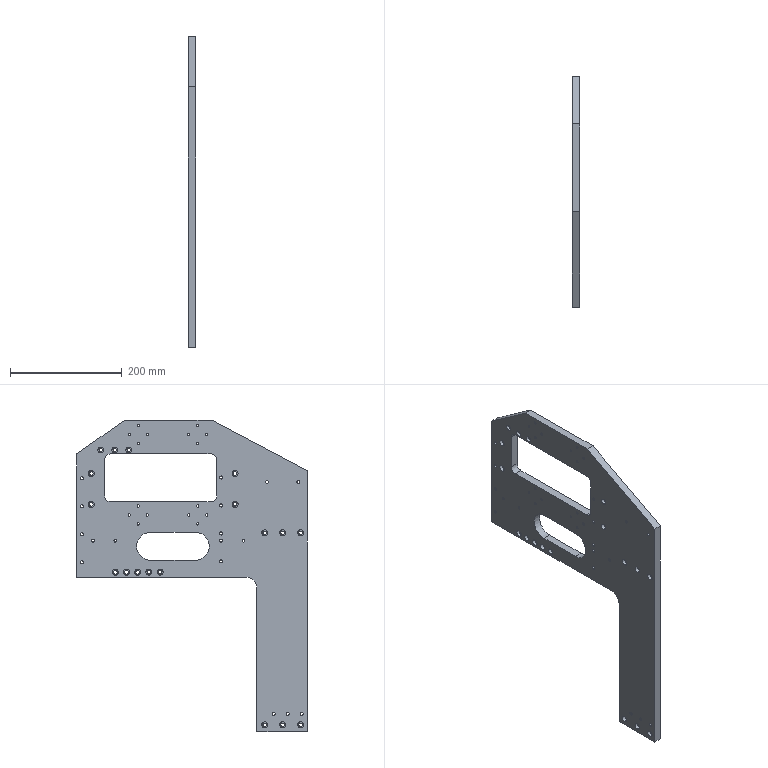Part | STEP file | support plate 13_SUS304 | 1 solid | 212 faces | box 14 x 412 x 556 mm | volume 1475012 mm3 | cylinder 167 | plane 45 | commonest cylinder face diameters 4.2 x32 6.6 x30 11 x30 5.5 x28 10 x28 5 x12